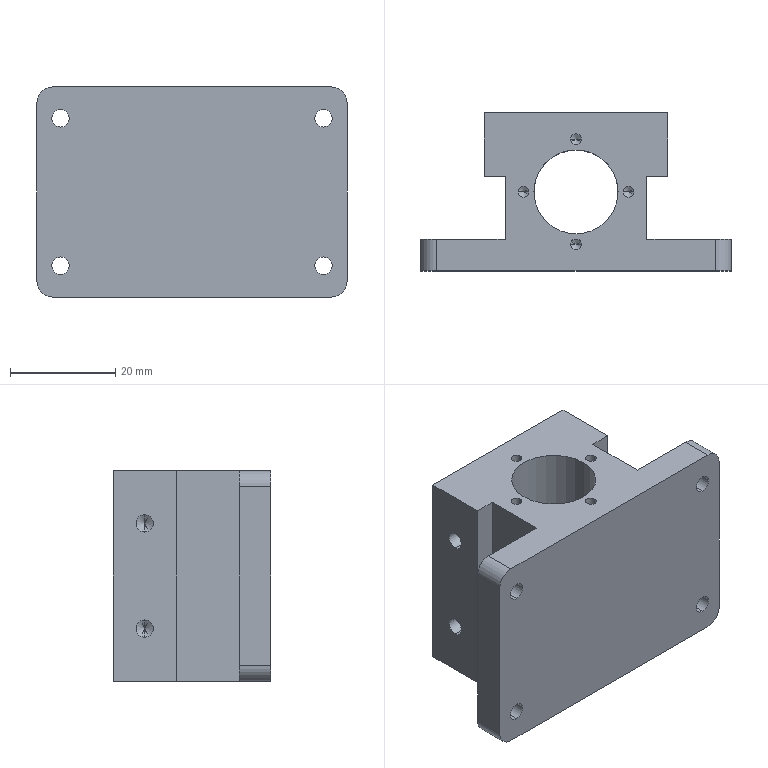Part | STEP file | Guide fixing seat | 1 solid | 60 faces | box 59 x 30 x 40 mm | volume 35183 mm3 | cylinder 30 | cone 16 | plane 14 | commonest cylinder face diameters 3.3 x16 2.05 x8 6 x4 16 x2